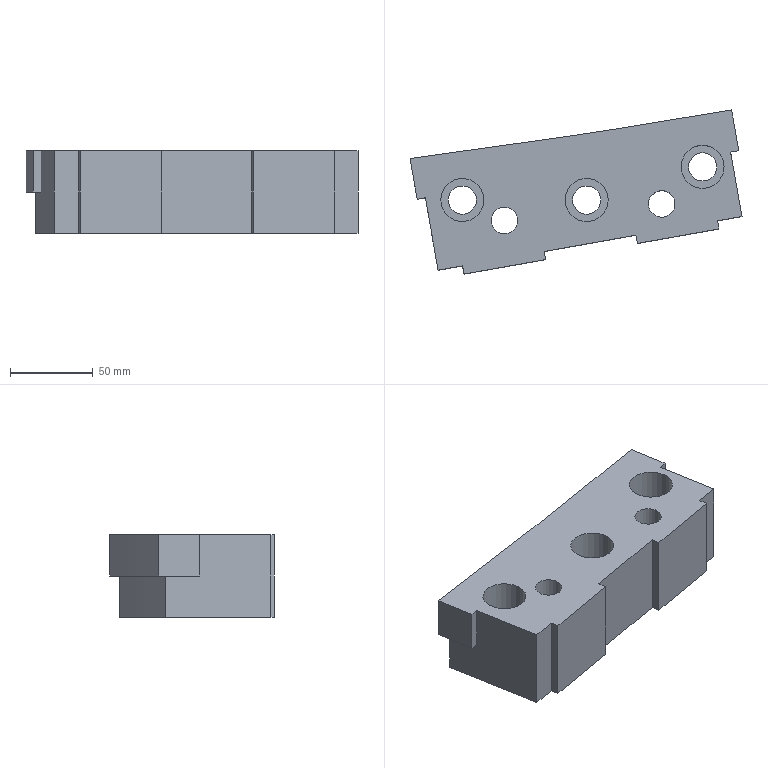Part | NX | features solid 2 | 1 solid | 31 faces | box 200.425 x 99.072 x 50 mm | volume 548993 mm3 | plane 21 | cylinder 8 | spline 2 | commonest cylinder face diameters 17 x3 26 x3 16 x2
STEP:
#1=CARTESIAN_POINT('',(8.477,507.421,0.));
#2=VERTEX_POINT('',#1);
#3=CARTESIAN_POINT('',(0.477,507.421,0.));
#4=DIRECTION('',(0.,0.,1.));
#5=DIRECTION('',(1.,0.,0.));
#6=AXIS2_PLACEMENT_3D('',#3,#4,#5);
#7=CIRCLE('',#6,8.);
#8=EDGE_CURVE('',#2,#2,#7,.T.);
#9=ORIENTED_EDGE('',*,*,#8,.F.);
#10=EDGE_LOOP('',(#9));
#11=FACE_BOUND('',#10,.T.);
#12=CARTESIAN_POINT('',(103.477,517.421,0.));
#13=VERTEX_POINT('',#12);
#14=CARTESIAN_POINT('',(95.477,517.421,0.));
#15=DIRECTION('',(0.,0.,1.));
#16=DIRECTION('',(1.,0.,0.));
#17=AXIS2_PLACEMENT_3D('',#14,#15,#16);
#18=CIRCLE('',#17,8.);
#19=EDGE_CURVE('',#13,#13,#18,.T.);
#20=ORIENTED_EDGE('',*,*,#19,.F.);
#21=EDGE_LOOP('',(#20));
#22=FACE_BOUND('',#21,.T.);
#23=CARTESIAN_POINT('',(-52.15,520.238,0.));
#24=VERTEX_POINT('',#23);
#25=CARTESIAN_POINT('',(-47.226,521.106,0.));
#26=VERTEX_POINT('',#25);
#27=CARTESIAN_POINT('',(-57.074,519.37,0.));
#28=DIRECTION('',(0.9848,0.1736,0.));
#29=VECTOR('',#28,1000.);
#30=LINE('',#27,#29);
#31=EDGE_CURVE('',#24,#26,#30,.T.);
#32=ORIENTED_EDGE('',*,*,#31,.T.);
#33=CARTESIAN_POINT('',(-39.523,477.421,0.));
#34=VERTEX_POINT('',#33);
#35=CARTESIAN_POINT('',(-39.523,477.421,0.));
#36=DIRECTION('',(-0.1736,0.9848,0.));
#37=VECTOR('',#36,1000.);
#38=LINE('',#35,#37);
#39=EDGE_CURVE('',#34,#26,#38,.T.);
#40=ORIENTED_EDGE('',*,*,#39,.F.);
#41=CARTESIAN_POINT('',(-24.751,480.026,0.));
#42=VERTEX_POINT('',#41);
#43=CARTESIAN_POINT('',(148.858,510.637,0.));
#44=DIRECTION('',(-0.9848,-0.1736,0.));
#45=VECTOR('',#44,1000.);
#46=LINE('',#43,#45);
#47=EDGE_CURVE('',#42,#34,#46,.T.);
#48=ORIENTED_EDGE('',*,*,#47,.F.);
#49=CARTESIAN_POINT('',(-23.883,475.101,0.));
#50=VERTEX_POINT('',#49);
#51=CARTESIAN_POINT('',(-24.751,480.026,0.));
#52=DIRECTION('',(0.1736,-0.9848,0.));
#53=VECTOR('',#52,1000.);
#54=LINE('',#51,#53);
#55=EDGE_CURVE('',#42,#50,#54,.T.);
#56=ORIENTED_EDGE('',*,*,#55,.T.);
#57=CARTESIAN_POINT('',(25.358,483.784,0.));
#58=VERTEX_POINT('',#57);
#59=CARTESIAN_POINT('',(25.358,483.784,0.));
#60=DIRECTION('',(-0.9848,-0.1736,0.));
#61=VECTOR('',#60,1000.);
#62=LINE('',#59,#61);
#63=EDGE_CURVE('',#58,#50,#62,.T.);
#64=ORIENTED_EDGE('',*,*,#63,.F.);
#65=CARTESIAN_POINT('',(24.49,488.708,0.));
#66=VERTEX_POINT('',#65);
#67=CARTESIAN_POINT('',(24.49,488.708,0.));
#68=DIRECTION('',(0.1736,-0.9848,0.));
#69=VECTOR('',#68,1000.);
#70=LINE('',#67,#69);
#71=EDGE_CURVE('',#66,#58,#70,.T.);
#72=ORIENTED_EDGE('',*,*,#71,.F.);
#73=CARTESIAN_POINT('',(79.921,498.482,0.));
#74=VERTEX_POINT('',#73);
#75=CARTESIAN_POINT('',(148.858,510.637,0.));
#76=DIRECTION('',(-0.9848,-0.1736,0.));
#77=VECTOR('',#76,1000.);
#78=LINE('',#75,#77);
#79=EDGE_CURVE('',#74,#66,#78,.T.);
#80=ORIENTED_EDGE('',*,*,#79,.F.);
#81=CARTESIAN_POINT('',(80.79,493.558,0.));
#82=VERTEX_POINT('',#81);
#83=CARTESIAN_POINT('',(79.921,498.482,0.));
#84=DIRECTION('',(0.1736,-0.9848,0.));
#85=VECTOR('',#84,1000.);
#86=LINE('',#83,#85);
#87=EDGE_CURVE('',#74,#82,#86,.T.);
#88=ORIENTED_EDGE('',*,*,#87,.T.);
#89=CARTESIAN_POINT('',(130.03,502.24,0.));
#90=VERTEX_POINT('',#89);
#91=CARTESIAN_POINT('',(144.802,504.845,0.));
#92=DIRECTION('',(-0.9848,-0.1736,0.));
#93=VECTOR('',#92,1000.);
#94=LINE('',#91,#93);
#95=EDGE_CURVE('',#90,#82,#94,.T.);
#96=ORIENTED_EDGE('',*,*,#95,.F.);
#97=CARTESIAN_POINT('',(129.162,507.164,0.));
#98=VERTEX_POINT('',#97);
#99=CARTESIAN_POINT('',(129.162,507.164,0.));
#100=DIRECTION('',(0.1736,-0.9848,0.));
#101=VECTOR('',#100,1000.);
#102=LINE('',#99,#101);
#103=EDGE_CURVE('',#98,#90,#102,.T.);
#104=ORIENTED_EDGE('',*,*,#103,.F.);
#105=CARTESIAN_POINT('',(143.934,509.769,0.));
#106=VERTEX_POINT('',#105);
#107=CARTESIAN_POINT('',(148.858,510.637,0.));
#108=DIRECTION('',(-0.9848,-0.1736,0.));
#109=VECTOR('',#108,1000.);
#110=LINE('',#107,#109);
#111=EDGE_CURVE('',#106,#98,#110,.T.);
#112=ORIENTED_EDGE('',*,*,#111,.F.);
#113=CARTESIAN_POINT('',(137.072,548.685,0.));
#114=VERTEX_POINT('',#113);
#115=CARTESIAN_POINT('',(143.934,509.769,0.));
#116=DIRECTION('',(-0.1736,0.9848,0.));
#117=VECTOR('',#116,1000.);
#118=LINE('',#115,#117);
#119=EDGE_CURVE('',#106,#114,#118,.T.);
#120=ORIENTED_EDGE('',*,*,#119,.T.);
#121=CARTESIAN_POINT('',(141.996,549.553,0.));
#122=VERTEX_POINT('',#121);
#123=CARTESIAN_POINT('',(146.92,550.422,0.));
#124=DIRECTION('',(-0.9848,-0.1736,0.));
#125=VECTOR('',#124,1000.);
#126=LINE('',#123,#125);
#127=EDGE_CURVE('',#122,#114,#126,.T.);
#128=ORIENTED_EDGE('',*,*,#127,.F.);
#129=CARTESIAN_POINT('',(137.655,574.174,0.));
#130=VERTEX_POINT('',#129);
#131=CARTESIAN_POINT('',(148.858,510.637,0.));
#132=DIRECTION('',(-0.1736,0.9848,0.));
#133=VECTOR('',#132,1000.);
#134=LINE('',#131,#133);
#135=EDGE_CURVE('',#122,#130,#134,.T.);
#136=ORIENTED_EDGE('',*,*,#135,.T.);
#137=CARTESIAN_POINT('',(-56.491,544.858,0.));
#138=VERTEX_POINT('',#137);
#139=CARTESIAN_POINT('',(137.655,574.174,0.));
#140=CARTESIAN_POINT('',(129.756,572.971,0.));
#141=CARTESIAN_POINT('',(112.276,570.118,0.));
#142=CARTESIAN_POINT('',(85.244,565.431,0.));
#143=CARTESIAN_POINT('',(56.452,560.795,0.));
#144=CARTESIAN_POINT('',(27.599,556.541,0.));
#145=CARTESIAN_POINT('',(-1.295,552.585,0.));
#146=CARTESIAN_POINT('',(-29.34,548.798,0.));
#147=CARTESIAN_POINT('',(-47.728,546.145,0.));
#148=CARTESIAN_POINT('',(-56.491,544.858,0.));
#149=B_SPLINE_CURVE_WITH_KNOTS('',3,(#139,#140,#141,#142,#143,#144,#145,#146,#147,#148),.UNSPECIFIED.,.F.,.F.,(4,1,1,1,1,1,1,4),(0.,0.1221,0.2706,0.4191,0.5676,0.7162,0.8647,1.),.UNSPECIFIED.);
#150=EDGE_CURVE('',#130,#138,#149,.T.);
#151=ORIENTED_EDGE('',*,*,#150,.T.);
#152=CARTESIAN_POINT('',(-44.447,476.553,0.));
#153=DIRECTION('',(-0.1736,0.9848,0.));
#154=VECTOR('',#153,1000.);
#155=LINE('',#152,#154);
#156=EDGE_CURVE('',#24,#138,#155,.T.);
#157=ORIENTED_EDGE('',*,*,#156,.F.);
#158=EDGE_LOOP('',(#32,#40,#48,#56,#64,#72,#80,#88,#96,#104,#112,#120,#128,#136,#151,#157));
#159=FACE_BOUND('',#158,.T.);
#160=CARTESIAN_POINT('',(63.122,519.794,0.));
#161=VERTEX_POINT('',#160);
#162=CARTESIAN_POINT('',(50.122,519.794,0.));
#163=DIRECTION('',(0.,0.,1.));
#164=DIRECTION('',(1.,0.,0.));
#165=AXIS2_PLACEMENT_3D('',#162,#163,#164);
#166=CIRCLE('',#165,13.);
#167=EDGE_CURVE('',#161,#161,#166,.T.);
#168=ORIENTED_EDGE('',*,*,#167,.F.);
#169=EDGE_LOOP('',(#168));
#170=FACE_BOUND('',#169,.T.);
#171=CARTESIAN_POINT('',(133.122,539.794,0.));
#172=VERTEX_POINT('',#171);
#173=CARTESIAN_POINT('',(120.122,539.794,0.));
#174=DIRECTION('',(0.,0.,1.));
#175=DIRECTION('',(1.,0.,0.));
#176=AXIS2_PLACEMENT_3D('',#173,#174,#175);
#177=CIRCLE('',#176,13.);
#178=EDGE_CURVE('',#172,#172,#177,.T.);
#179=ORIENTED_EDGE('',*,*,#178,.F.);
#180=EDGE_LOOP('',(#179));
#181=FACE_BOUND('',#180,.T.);
#182=CARTESIAN_POINT('',(-37.878,519.794,0.));
#183=VERTEX_POINT('',#182);
#184=CARTESIAN_POINT('',(-24.878,519.794,0.));
#185=DIRECTION('',(0.,0.,-1.));
#186=DIRECTION('',(-1.,0.,0.));
#187=AXIS2_PLACEMENT_3D('',#184,#185,#186);
#188=CIRCLE('',#187,13.);
#189=EDGE_CURVE('',#183,#183,#188,.T.);
#190=ORIENTED_EDGE('',*,*,#189,.T.);
#191=EDGE_LOOP('',(#190));
#192=FACE_BOUND('',#191,.T.);
#193=CARTESIAN_POINT('',(-40.143,-832.432,0.));
#194=DIRECTION('',(0.,0.,1.));
#195=DIRECTION('',(0.9962,-0.08716,0.));
#196=AXIS2_PLACEMENT_3D('',#193,#194,#195);
#197=PLANE('',#196);
#198=ADVANCED_FACE('',(#11,#22,#159,#170,#181,#192),#197,.T.);
#199=CARTESIAN_POINT('',(-52.15,520.238,-25.));
#200=VERTEX_POINT('',#199);
#201=CARTESIAN_POINT('',(-47.226,521.106,-25.));
#202=VERTEX_POINT('',#201);
#203=CARTESIAN_POINT('',(-57.074,519.37,-25.));
#204=DIRECTION('',(0.9848,0.1736,0.));
#205=VECTOR('',#204,1000.);
#206=LINE('',#203,#205);
#207=EDGE_CURVE('',#200,#202,#206,.T.);
#208=ORIENTED_EDGE('',*,*,#207,.F.);
#209=CARTESIAN_POINT('',(-56.491,544.858,-25.));
#210=VERTEX_POINT('',#209);
#211=CARTESIAN_POINT('',(-44.447,476.553,-25.));
#212=DIRECTION('',(0.1736,-0.9848,0.));
#213=VECTOR('',#212,1000.);
#214=LINE('',#211,#213);
#215=EDGE_CURVE('',#210,#200,#214,.T.);
#216=ORIENTED_EDGE('',*,*,#215,.F.);
#217=CARTESIAN_POINT('',(137.655,574.174,-25.));
#218=VERTEX_POINT('',#217);
#219=CARTESIAN_POINT('',(137.655,574.174,-25.));
#220=CARTESIAN_POINT('',(129.756,572.971,-25.));
#221=CARTESIAN_POINT('',(112.276,570.118,-25.));
#222=CARTESIAN_POINT('',(85.244,565.431,-25.));
#223=CARTESIAN_POINT('',(56.452,560.795,-25.));
#224=CARTESIAN_POINT('',(27.599,556.541,-25.));
#225=CARTESIAN_POINT('',(-1.295,552.585,-25.));
#226=CARTESIAN_POINT('',(-29.34,548.798,-25.));
#227=CARTESIAN_POINT('',(-47.728,546.145,-25.));
#228=CARTESIAN_POINT('',(-56.491,544.858,-25.));
#229=B_SPLINE_CURVE_WITH_KNOTS('',3,(#219,#220,#221,#222,#223,#224,#225,#226,#227,#228),.UNSPECIFIED.,.F.,.F.,(4,1,1,1,1,1,1,4),(0.,0.1221,0.2706,0.4191,0.5676,0.7162,0.8647,1.),.UNSPECIFIED.);
#230=EDGE_CURVE('',#210,#218,#229,.F.);
#231=ORIENTED_EDGE('',*,*,#230,.T.);
#232=CARTESIAN_POINT('',(141.996,549.553,-25.));
#233=VERTEX_POINT('',#232);
#234=CARTESIAN_POINT('',(148.858,510.637,-25.));
#235=DIRECTION('',(0.1736,-0.9848,0.));
#236=VECTOR('',#235,1000.);
#237=LINE('',#234,#236);
#238=EDGE_CURVE('',#218,#233,#237,.T.);
#239=ORIENTED_EDGE('',*,*,#238,.T.);
#240=CARTESIAN_POINT('',(137.072,548.685,-25.));
#241=VERTEX_POINT('',#240);
#242=CARTESIAN_POINT('',(146.92,550.422,-25.));
#243=DIRECTION('',(-0.9848,-0.1736,0.));
#244=VECTOR('',#243,1000.);
#245=LINE('',#242,#244);
#246=EDGE_CURVE('',#233,#241,#245,.T.);
#247=ORIENTED_EDGE('',*,*,#246,.T.);
#248=CARTESIAN_POINT('',(133.581,568.485,-25.));
#249=VERTEX_POINT('',#248);
#250=CARTESIAN_POINT('',(143.934,509.769,-25.));
#251=DIRECTION('',(0.1736,-0.9848,0.));
#252=VECTOR('',#251,1000.);
#253=LINE('',#250,#252);
#254=EDGE_CURVE('',#241,#249,#253,.F.);
#255=ORIENTED_EDGE('',*,*,#254,.T.);
#256=CARTESIAN_POINT('',(-50.673,540.656,-25.));
#257=VERTEX_POINT('',#256);
#258=CARTESIAN_POINT('',(133.581,568.485,-25.));
#259=CARTESIAN_POINT('',(118.304,566.095,-25.));
#260=CARTESIAN_POINT('',(87.745,560.699,-25.));
#261=CARTESIAN_POINT('',(41.601,553.395,-25.));
#262=CARTESIAN_POINT('',(-4.622,547.104,-25.));
#263=CARTESIAN_POINT('',(-35.327,542.893,-25.));
#264=CARTESIAN_POINT('',(-50.673,540.656,-25.));
#265=B_SPLINE_CURVE_WITH_KNOTS('',3,(#258,#259,#260,#261,#262,#263,#264),.UNSPECIFIED.,.F.,.F.,(4,1,1,1,4),(0.02498,0.2622,0.4994,0.7366,0.9738),.UNSPECIFIED.);
#266=EDGE_CURVE('',#249,#257,#265,.T.);
#267=ORIENTED_EDGE('',*,*,#266,.T.);
#268=CARTESIAN_POINT('',(-39.523,477.421,-25.));
#269=DIRECTION('',(0.1736,-0.9848,0.));
#270=VECTOR('',#269,1000.);
#271=LINE('',#268,#270);
#272=EDGE_CURVE('',#202,#257,#271,.F.);
#273=ORIENTED_EDGE('',*,*,#272,.F.);
#274=EDGE_LOOP('',(#208,#216,#231,#239,#247,#255,#267,#273));
#275=FACE_BOUND('',#274,.T.);
#276=CARTESIAN_POINT('',(-56.491,544.858,-25.));
#277=DIRECTION('',(0.,0.,-1.));
#278=DIRECTION('',(-0.9962,0.08716,0.));
#279=AXIS2_PLACEMENT_3D('',#276,#277,#278);
#280=PLANE('',#279);
#281=ADVANCED_FACE('',(#275),#280,.T.);
#282=ORIENTED_EDGE('',*,*,#135,.F.);
#283=CARTESIAN_POINT('',(141.996,549.553,-50.));
#284=DIRECTION('',(0.,0.,-1.));
#285=VECTOR('',#284,1000.);
#286=LINE('',#283,#285);
#287=EDGE_CURVE('',#122,#233,#286,.T.);
#288=ORIENTED_EDGE('',*,*,#287,.T.);
#289=ORIENTED_EDGE('',*,*,#238,.F.);
#290=CARTESIAN_POINT('',(137.655,574.174,-50.));
#291=DIRECTION('',(0.,0.,1.));
#292=VECTOR('',#291,1000.);
#293=LINE('',#290,#292);
#294=EDGE_CURVE('',#218,#130,#293,.T.);
#295=ORIENTED_EDGE('',*,*,#294,.T.);
#296=EDGE_LOOP('',(#282,#288,#289,#295));
#297=FACE_BOUND('',#296,.T.);
#298=CARTESIAN_POINT('',(148.858,510.637,-50.));
#299=DIRECTION('',(0.9848,0.1736,0.));
#300=DIRECTION('',(-0.1736,0.9848,0.));
#301=AXIS2_PLACEMENT_3D('',#298,#299,#300);
#302=PLANE('',#301);
#303=ADVANCED_FACE('',(#297),#302,.T.);
#304=CARTESIAN_POINT('',(143.934,509.769,-50.));
#305=VERTEX_POINT('',#304);
#306=CARTESIAN_POINT('',(143.934,509.769,-50.));
#307=DIRECTION('',(0.,0.,1.));
#308=VECTOR('',#307,1000.);
#309=LINE('',#306,#308);
#310=EDGE_CURVE('',#305,#106,#309,.T.);
#311=ORIENTED_EDGE('',*,*,#310,.T.);
#312=ORIENTED_EDGE('',*,*,#111,.T.);
#313=CARTESIAN_POINT('',(129.162,507.164,-50.));
#314=VERTEX_POINT('',#313);
#315=CARTESIAN_POINT('',(129.162,507.164,-50.));
#316=DIRECTION('',(0.,0.,1.));
#317=VECTOR('',#316,1000.);
#318=LINE('',#315,#317);
#319=EDGE_CURVE('',#314,#98,#318,.T.);
#320=ORIENTED_EDGE('',*,*,#319,.F.);
#321=CARTESIAN_POINT('',(148.858,510.637,-50.));
#322=DIRECTION('',(-0.9848,-0.1736,0.));
#323=VECTOR('',#322,1000.);
#324=LINE('',#321,#323);
#325=EDGE_CURVE('',#305,#314,#324,.T.);
#326=ORIENTED_EDGE('',*,*,#325,.F.);
#327=EDGE_LOOP('',(#311,#312,#320,#326));
#328=FACE_BOUND('',#327,.T.);
#329=CARTESIAN_POINT('',(148.858,510.637,-50.));
#330=DIRECTION('',(-0.1736,0.9848,0.));
#331=DIRECTION('',(-0.9848,-0.1736,0.));
#332=AXIS2_PLACEMENT_3D('',#329,#330,#331);
#333=PLANE('',#332);
#334=ADVANCED_FACE('',(#328),#333,.F.);
#335=CARTESIAN_POINT('',(8.477,507.421,-50.));
#336=VERTEX_POINT('',#335);
#337=CARTESIAN_POINT('',(0.477,507.421,-50.));
#338=DIRECTION('',(0.,0.,1.));
#339=DIRECTION('',(1.,0.,0.));
#340=AXIS2_PLACEMENT_3D('',#337,#338,#339);
#341=CIRCLE('',#340,8.);
#342=EDGE_CURVE('',#336,#336,#341,.T.);
#343=ORIENTED_EDGE('',*,*,#342,.T.);
#344=EDGE_LOOP('',(#343));
#345=FACE_BOUND('',#344,.T.);
#346=CARTESIAN_POINT('',(103.477,517.421,-50.));
#347=VERTEX_POINT('',#346);
#348=CARTESIAN_POINT('',(95.477,517.421,-50.));
#349=DIRECTION('',(0.,0.,1.));
#350=DIRECTION('',(1.,0.,0.));
#351=AXIS2_PLACEMENT_3D('',#348,#349,#350);
#352=CIRCLE('',#351,8.);
#353=EDGE_CURVE('',#347,#347,#352,.T.);
#354=ORIENTED_EDGE('',*,*,#353,.T.);
#355=EDGE_LOOP('',(#354));
#356=FACE_BOUND('',#355,.T.);
#357=CARTESIAN_POINT('',(133.581,568.485,-50.));
#358=VERTEX_POINT('',#357);
#359=CARTESIAN_POINT('',(132.49,574.671,-50.));
#360=DIRECTION('',(-0.1736,0.9848,0.));
#361=VECTOR('',#360,1000.);
#362=LINE('',#359,#361);
#363=EDGE_CURVE('',#305,#358,#362,.T.);
#364=ORIENTED_EDGE('',*,*,#363,.F.);
#365=ORIENTED_EDGE('',*,*,#325,.T.);
#366=CARTESIAN_POINT('',(130.03,502.24,-50.));
#367=VERTEX_POINT('',#366);
#368=CARTESIAN_POINT('',(129.162,507.164,-50.));
#369=DIRECTION('',(0.1736,-0.9848,0.));
#370=VECTOR('',#369,1000.);
#371=LINE('',#368,#370);
#372=EDGE_CURVE('',#314,#367,#371,.T.);
#373=ORIENTED_EDGE('',*,*,#372,.T.);
#374=CARTESIAN_POINT('',(80.79,493.558,-50.));
#375=VERTEX_POINT('',#374);
#376=CARTESIAN_POINT('',(144.802,504.845,-50.));
#377=DIRECTION('',(-0.9848,-0.1736,0.));
#378=VECTOR('',#377,1000.);
#379=LINE('',#376,#378);
#380=EDGE_CURVE('',#367,#375,#379,.T.);
#381=ORIENTED_EDGE('',*,*,#380,.T.);
#382=CARTESIAN_POINT('',(79.921,498.482,-50.));
#383=VERTEX_POINT('',#382);
#384=CARTESIAN_POINT('',(79.921,498.482,-50.));
#385=DIRECTION('',(0.1736,-0.9848,0.));
#386=VECTOR('',#385,1000.);
#387=LINE('',#384,#386);
#388=EDGE_CURVE('',#383,#375,#387,.T.);
#389=ORIENTED_EDGE('',*,*,#388,.F.);
#390=CARTESIAN_POINT('',(24.49,488.708,-50.));
#391=VERTEX_POINT('',#390);
#392=CARTESIAN_POINT('',(148.858,510.637,-50.));
#393=DIRECTION('',(-0.9848,-0.1736,0.));
#394=VECTOR('',#393,1000.);
#395=LINE('',#392,#394);
#396=EDGE_CURVE('',#383,#391,#395,.T.);
#397=ORIENTED_EDGE('',*,*,#396,.T.);
#398=CARTESIAN_POINT('',(25.358,483.784,-50.));
#399=VERTEX_POINT('',#398);
#400=CARTESIAN_POINT('',(24.49,488.708,-50.));
#401=DIRECTION('',(0.1736,-0.9848,0.));
#402=VECTOR('',#401,1000.);
#403=LINE('',#400,#402);
#404=EDGE_CURVE('',#391,#399,#403,.T.);
#405=ORIENTED_EDGE('',*,*,#404,.T.);
#406=CARTESIAN_POINT('',(-23.883,475.101,-50.));
#407=VERTEX_POINT('',#406);
#408=CARTESIAN_POINT('',(25.358,483.784,-50.));
#409=DIRECTION('',(-0.9848,-0.1736,0.));
#410=VECTOR('',#409,1000.);
#411=LINE('',#408,#410);
#412=EDGE_CURVE('',#399,#407,#411,.T.);
#413=ORIENTED_EDGE('',*,*,#412,.T.);
#414=CARTESIAN_POINT('',(-24.751,480.026,-50.));
#415=VERTEX_POINT('',#414);
#416=CARTESIAN_POINT('',(-24.751,480.026,-50.));
#417=DIRECTION('',(0.1736,-0.9848,0.));
#418=VECTOR('',#417,1000.);
#419=LINE('',#416,#418);
#420=EDGE_CURVE('',#415,#407,#419,.T.);
#421=ORIENTED_EDGE('',*,*,#420,.F.);
#422=CARTESIAN_POINT('',(-39.523,477.421,-50.));
#423=VERTEX_POINT('',#422);
#424=CARTESIAN_POINT('',(148.858,510.637,-50.));
#425=DIRECTION('',(-0.9848,-0.1736,0.));
#426=VECTOR('',#425,1000.);
#427=LINE('',#424,#426);
#428=EDGE_CURVE('',#415,#423,#427,.T.);
#429=ORIENTED_EDGE('',*,*,#428,.T.);
#430=CARTESIAN_POINT('',(-50.673,540.656,-50.));
#431=VERTEX_POINT('',#430);
#432=CARTESIAN_POINT('',(-50.967,542.323,-50.));
#433=DIRECTION('',(-0.1736,0.9848,0.));
#434=VECTOR('',#433,1000.);
#435=LINE('',#432,#434);
#436=EDGE_CURVE('',#423,#431,#435,.T.);
#437=ORIENTED_EDGE('',*,*,#436,.T.);
#438=CARTESIAN_POINT('',(-50.673,540.656,-50.));
#439=CARTESIAN_POINT('',(-48.626,540.955,-50.));
#440=CARTESIAN_POINT('',(-44.596,541.539,-50.));
#441=CARTESIAN_POINT('',(-39.713,542.24,-50.));
#442=CARTESIAN_POINT('',(-35.901,542.783,-50.));
#443=CARTESIAN_POINT('',(-33.086,543.181,-50.));
#444=CARTESIAN_POINT('',(-30.79,543.504,-50.));
#445=CARTESIAN_POINT('',(-29.182,543.729,-50.));
#446=CARTESIAN_POINT('',(-28.302,543.852,-50.));
#447=CARTESIAN_POINT('',(-27.552,543.956,-50.));
#448=CARTESIAN_POINT('',(-27.161,544.011,-50.));
#449=CARTESIAN_POINT('',(-26.486,544.104,-50.));
#450=CARTESIAN_POINT('',(-25.31,544.267,-50.));
#451=CARTESIAN_POINT('',(-23.436,544.526,-50.));
#452=CARTESIAN_POINT('',(-20.942,544.869,-50.));
#453=CARTESIAN_POINT('',(-17.266,545.373,-50.));
#454=CARTESIAN_POINT('',(-13.079,545.945,-50.));
#455=CARTESIAN_POINT('',(-8.95,546.508,-50.));
#456=CARTESIAN_POINT('',(-6.48,546.844,-50.));
#457=CARTESIAN_POINT('',(-3.855,547.2,-50.));
#458=CARTESIAN_POINT('',(-0.8949,547.603,-50.));
#459=CARTESIAN_POINT('',(3.851,548.25,-50.));
#460=CARTESIAN_POINT('',(11.737,549.332,-50.));
#461=CARTESIAN_POINT('',(19.972,550.475,-50.));
#462=CARTESIAN_POINT('',(27.393,551.518,-50.));
#463=CARTESIAN_POINT('',(31.695,552.13,-50.));
#464=CARTESIAN_POINT('',(34.937,552.595,-50.));
#465=CARTESIAN_POINT('',(37.264,552.932,-50.));
#466=CARTESIAN_POINT('',(39.13,553.203,-50.));
#467=CARTESIAN_POINT('',(40.371,553.385,-50.));
#468=CARTESIAN_POINT('',(41.1,553.492,-50.));
#469=CARTESIAN_POINT('',(41.55,553.558,-50.));
#470=CARTESIAN_POINT('',(42.339,553.675,-50.));
#471=CARTESIAN_POINT('',(43.272,553.812,-50.));
#472=CARTESIAN_POINT('',(44.961,554.063,-50.));
#473=CARTESIAN_POINT('',(47.345,554.419,-50.));
#474=CARTESIAN_POINT('',(50.219,554.851,-50.));
#475=CARTESIAN_POINT('',(54.048,555.433,-50.));
#476=CARTESIAN_POINT('',(58.838,556.169,-50.));
#477=CARTESIAN_POINT('',(66.506,557.368,-50.));
#478=CARTESIAN_POINT('',(76.095,558.903,-50.));
#479=CARTESIAN_POINT('',(87.637,560.814,-50.));
#480=CARTESIAN_POINT('',(97.202,562.433,-50.));
#481=CARTESIAN_POINT('',(104.843,563.732,-50.));
#482=CARTESIAN_POINT('',(110.63,564.726,-50.));
#483=CARTESIAN_POINT('',(116.194,565.673,-50.));
#484=CARTESIAN_POINT('',(123.825,566.938,-50.));
#485=CARTESIAN_POINT('',(129.643,567.869,-50.));
#486=CARTESIAN_POINT('',(133.581,568.485,-50.));
#487=B_SPLINE_CURVE_WITH_KNOTS('',3,(#438,#439,#440,#441,#442,#443,#444,#445,#446,#447,#448,#449,#450,#451,#452,#453,#454,#455,#456,#457,#458,#459,#460,#461,#462,#463,#464,#465,#466,#467,#468,#469,#470,#471,#472,#473,#474,#475,#476,#477,#478,#479,#480,#481,#482,#483,#484,#485,#486),.UNSPECIFIED.,.F.,.F.,(4,1,1,1,1,1,1,1,1,1,1,1,1,1,1,1,1,1,1,1,1,1,1,1,1,1,1,1,1,1,1,1,1,1,1,1,1,1,1,1,1,1,1,1,1,1,4),(0.,0.03125,0.0625,0.07812,0.09375,0.1094,0.1172,0.1211,0.125,0.1289,0.1328,0.1406,0.1562,0.1719,0.1875,0.2188,0.2344,0.2422,0.25,0.2656,0.2812,0.3125,0.375,0.4062,0.4375,0.4531,0.4688,0.4844,0.4922,0.4961,0.5,0.5039,0.5078,0.5156,0.5312,0.5469,0.5625,0.5938,0.625,0.6875,0.75,0.8125,0.8438,0.875,0.9062,0.9375,1.),.UNSPECIFIED.);
#488=EDGE_CURVE('',#358,#431,#487,.F.);
#489=ORIENTED_EDGE('',*,*,#488,.F.);
#490=EDGE_LOOP('',(#364,#365,#373,#381,#389,#397,#405,#413,#421,#429,#437,#489));
#491=FACE_BOUND('',#490,.T.);
#492=CARTESIAN_POINT('',(41.622,519.794,-50.));
#493=VERTEX_POINT('',#492);
#494=CARTESIAN_POINT('',(50.122,519.794,-50.));
#495=DIRECTION('',(0.,0.,-1.));
#496=DIRECTION('',(-1.,0.,0.));
#497=AXIS2_PLACEMENT_3D('',#494,#495,#496);
#498=CIRCLE('',#497,8.5);
#499=EDGE_CURVE('',#493,#493,#498,.T.);
#500=ORIENTED_EDGE('',*,*,#499,.F.);
#501=EDGE_LOOP('',(#500));
#502=FACE_BOUND('',#501,.T.);
#503=CARTESIAN_POINT('',(111.622,539.794,-50.));
#504=VERTEX_POINT('',#503);
#505=CARTESIAN_POINT('',(120.122,539.794,-50.));
#506=DIRECTION('',(0.,0.,-1.));
#507=DIRECTION('',(-1.,0.,0.));
#508=AXIS2_PLACEMENT_3D('',#505,#506,#507);
#509=CIRCLE('',#508,8.5);
#510=EDGE_CURVE('',#504,#504,#509,.T.);
#511=ORIENTED_EDGE('',*,*,#510,.F.);
#512=EDGE_LOOP('',(#511));
#513=FACE_BOUND('',#512,.T.);
#514=CARTESIAN_POINT('',(-33.378,519.794,-50.));
#515=VERTEX_POINT('',#514);
#516=CARTESIAN_POINT('',(-24.878,519.794,-50.));
#517=DIRECTION('',(0.,0.,-1.));
#518=DIRECTION('',(-1.,0.,0.));
#519=AXIS2_PLACEMENT_3D('',#516,#517,#518);
#520=CIRCLE('',#519,8.5);
#521=EDGE_CURVE('',#515,#515,#520,.T.);
#522=ORIENTED_EDGE('',*,*,#521,.F.);
#523=EDGE_LOOP('',(#522));
#524=FACE_BOUND('',#523,.T.);
#525=CARTESIAN_POINT('',(-40.143,-832.432,-50.));
#526=DIRECTION('',(0.,0.,1.));
#527=DIRECTION('',(0.9962,-0.08716,0.));
#528=AXIS2_PLACEMENT_3D('',#525,#526,#527);
#529=PLANE('',#528);
#530=ADVANCED_FACE('',(#345,#356,#491,#502,#513,#524),#529,.F.);
#531=CARTESIAN_POINT('',(-11.878,519.794,-25.));
#532=VERTEX_POINT('',#531);
#533=CARTESIAN_POINT('',(-24.878,519.794,-25.));
#534=DIRECTION('',(0.,0.,1.));
#535=DIRECTION('',(1.,0.,0.));
#536=AXIS2_PLACEMENT_3D('',#533,#534,#535);
#537=CIRCLE('',#536,13.);
#538=EDGE_CURVE('',#532,#532,#537,.T.);
#539=ORIENTED_EDGE('',*,*,#538,.T.);
#540=EDGE_LOOP('',(#539));
#541=FACE_BOUND('',#540,.T.);
#542=CARTESIAN_POINT('',(-33.378,519.794,-25.));
#543=VERTEX_POINT('',#542);
#544=CARTESIAN_POINT('',(-24.878,519.794,-25.));
#545=DIRECTION('',(0.,0.,-1.));
#546=DIRECTION('',(-1.,0.,0.));
#547=AXIS2_PLACEMENT_3D('',#544,#545,#546);
#548=CIRCLE('',#547,8.5);
#549=EDGE_CURVE('',#543,#543,#548,.F.);
#550=ORIENTED_EDGE('',*,*,#549,.F.);
#551=EDGE_LOOP('',(#550));
#552=FACE_BOUND('',#551,.T.);
#553=CARTESIAN_POINT('',(-24.878,519.794,-25.));
#554=DIRECTION('',(0.,0.,-1.));
#555=DIRECTION('',(-1.,0.,0.));
#556=AXIS2_PLACEMENT_3D('',#553,#554,#555);
#557=PLANE('',#556);
#558=ADVANCED_FACE('',(#541,#552),#557,.F.);
#559=ORIENTED_EDGE('',*,*,#521,.T.);
#560=EDGE_LOOP('',(#559));
#561=FACE_BOUND('',#560,.T.);
#562=ORIENTED_EDGE('',*,*,#549,.T.);
#563=EDGE_LOOP('',(#562));
#564=FACE_BOUND('',#563,.T.);
#565=CARTESIAN_POINT('',(-24.878,519.794,-75.));
#566=DIRECTION('',(0.,0.,1.));
#567=DIRECTION('',(1.,0.,0.));
#568=AXIS2_PLACEMENT_3D('',#565,#566,#567);
#569=CYLINDRICAL_SURFACE('',#568,8.5);
#570=ADVANCED_FACE('',(#561,#564),#569,.F.);
#571=ORIENTED_EDGE('',*,*,#189,.F.);
#572=EDGE_LOOP('',(#571));
#573=FACE_BOUND('',#572,.T.);
#574=ORIENTED_EDGE('',*,*,#538,.F.);
#575=EDGE_LOOP('',(#574));
#576=FACE_BOUND('',#575,.T.);
#577=CARTESIAN_POINT('',(-24.878,519.794,-25.));
#578=DIRECTION('',(0.,0.,1.));
#579=DIRECTION('',(1.,0.,0.));
#580=AXIS2_PLACEMENT_3D('',#577,#578,#579);
#581=CYLINDRICAL_SURFACE('',#580,13.);
#582=ADVANCED_FACE('',(#573,#576),#581,.F.);
#583=ORIENTED_EDGE('',*,*,#215,.T.);
#584=CARTESIAN_POINT('',(-52.15,520.238,-50.));
#585=DIRECTION('',(0.,0.,1.));
#586=VECTOR('',#585,1000.);
#587=LINE('',#584,#586);
#588=EDGE_CURVE('',#200,#24,#587,.T.);
#589=ORIENTED_EDGE('',*,*,#588,.T.);
#590=ORIENTED_EDGE('',*,*,#156,.T.);
#591=CARTESIAN_POINT('',(-56.491,544.858,-50.));
#592=DIRECTION('',(0.,0.,1.));
#593=VECTOR('',#592,1000.);
#594=LINE('',#591,#593);
#595=EDGE_CURVE('',#210,#138,#594,.T.);
#596=ORIENTED_EDGE('',*,*,#595,.F.);
#597=EDGE_LOOP('',(#583,#589,#590,#596));
#598=FACE_BOUND('',#597,.T.);
#599=CARTESIAN_POINT('',(-44.447,476.553,-50.));
#600=DIRECTION('',(0.9848,0.1736,0.));
#601=DIRECTION('',(-0.1736,0.9848,0.));
#602=AXIS2_PLACEMENT_3D('',#599,#600,#601);
#603=PLANE('',#602);
#604=ADVANCED_FACE('',(#598),#603,.F.);
#605=ORIENTED_EDGE('',*,*,#230,.F.);
#606=ORIENTED_EDGE('',*,*,#595,.T.);
#607=ORIENTED_EDGE('',*,*,#150,.F.);
#608=ORIENTED_EDGE('',*,*,#294,.F.);
#609=EDGE_LOOP('',(#605,#606,#607,#608));
#610=FACE_BOUND('',#609,.T.);
#611=CARTESIAN_POINT('',(137.655,574.174,-25.));
#612=CARTESIAN_POINT('',(137.655,574.174,0.));
#613=CARTESIAN_POINT('',(121.479,571.711,-25.));
#614=CARTESIAN_POINT('',(121.479,571.711,0.));
#615=CARTESIAN_POINT('',(89.246,566.024,-25.));
#616=CARTESIAN_POINT('',(89.246,566.024,0.));
#617=CARTESIAN_POINT('',(40.765,558.301,-25.));
#618=CARTESIAN_POINT('',(40.765,558.301,0.));
#619=CARTESIAN_POINT('',(-7.885,551.726,-25.));
#620=CARTESIAN_POINT('',(-7.885,551.726,0.));
#621=CARTESIAN_POINT('',(-40.302,547.236,-25.));
#622=CARTESIAN_POINT('',(-40.302,547.236,0.));
#623=CARTESIAN_POINT('',(-56.491,544.858,-25.));
#624=CARTESIAN_POINT('',(-56.491,544.858,0.));
#625=B_SPLINE_SURFACE_WITH_KNOTS('',3,1,((#611,#612),(#613,#614),(#615,#616),(#617,#618),(#619,#620),(#621,#622),(#623,#624)),.SURF_OF_LINEAR_EXTRUSION.,.F.,.F.,.F.,(4,1,1,1,4),(2,2),(0.,0.25,0.5,0.75,1.),(0.,1.),.UNSPECIFIED.);
#626=ADVANCED_FACE('',(#610),#625,.T.);
#627=ORIENTED_EDGE('',*,*,#254,.F.);
#628=CARTESIAN_POINT('',(137.072,548.685,-50.));
#629=DIRECTION('',(0.,0.,1.));
#630=VECTOR('',#629,1000.);
#631=LINE('',#628,#630);
#632=EDGE_CURVE('',#241,#114,#631,.T.);
#633=ORIENTED_EDGE('',*,*,#632,.T.);
#634=ORIENTED_EDGE('',*,*,#119,.F.);
#635=ORIENTED_EDGE('',*,*,#310,.F.);
#636=ORIENTED_EDGE('',*,*,#363,.T.);
#637=CARTESIAN_POINT('',(133.581,568.485,-37.5));
#638=DIRECTION('',(0.,0.,-1.));
#639=VECTOR('',#638,1000.);
#640=LINE('',#637,#639);
#641=EDGE_CURVE('',#249,#358,#640,.T.);
#642=ORIENTED_EDGE('',*,*,#641,.F.);
#643=EDGE_LOOP('',(#627,#633,#634,#635,#636,#642));
#644=FACE_BOUND('',#643,.T.);
#645=CARTESIAN_POINT('',(143.934,509.769,-25.));
#646=DIRECTION('',(-0.9848,-0.1736,0.));
#647=DIRECTION('',(0.1736,-0.9848,0.));
#648=AXIS2_PLACEMENT_3D('',#645,#646,#647);
#649=PLANE('',#648);
#650=ADVANCED_FACE('',(#644),#649,.F.);
#651=ORIENTED_EDGE('',*,*,#436,.F.);
#652=CARTESIAN_POINT('',(-39.523,477.421,-50.));
#653=DIRECTION('',(0.,0.,1.));
#654=VECTOR('',#653,1000.);
#655=LINE('',#652,#654);
#656=EDGE_CURVE('',#423,#34,#655,.T.);
#657=ORIENTED_EDGE('',*,*,#656,.T.);
#658=ORIENTED_EDGE('',*,*,#39,.T.);
#659=CARTESIAN_POINT('',(-47.226,521.106,-50.));
#660=DIRECTION('',(0.,0.,1.));
#661=VECTOR('',#660,1000.);
#662=LINE('',#659,#661);
#663=EDGE_CURVE('',#202,#26,#662,.T.);
#664=ORIENTED_EDGE('',*,*,#663,.F.);
#665=ORIENTED_EDGE('',*,*,#272,.T.);
#666=CARTESIAN_POINT('',(-50.673,540.656,-37.5));
#667=DIRECTION('',(0.,0.,-1.));
#668=VECTOR('',#667,1000.);
#669=LINE('',#666,#668);
#670=EDGE_CURVE('',#257,#431,#669,.T.);
#671=ORIENTED_EDGE('',*,*,#670,.T.);
#672=EDGE_LOOP('',(#651,#657,#658,#664,#665,#671));
#673=FACE_BOUND('',#672,.T.);
#674=CARTESIAN_POINT('',(-39.523,477.421,-25.));
#675=DIRECTION('',(-0.9848,-0.1736,0.));
#676=DIRECTION('',(0.1736,-0.9848,0.));
#677=AXIS2_PLACEMENT_3D('',#674,#675,#676);
#678=PLANE('',#677);
#679=ADVANCED_FACE('',(#673),#678,.T.);
#680=ORIENTED_EDGE('',*,*,#266,.F.);
#681=ORIENTED_EDGE('',*,*,#641,.T.);
#682=ORIENTED_EDGE('',*,*,#488,.T.);
#683=ORIENTED_EDGE('',*,*,#670,.F.);
#684=EDGE_LOOP('',(#680,#681,#682,#683));
#685=FACE_BOUND('',#684,.T.);
#686=CARTESIAN_POINT('',(133.581,568.485,-25.));
#687=CARTESIAN_POINT('',(133.581,568.485,-50.));
#688=CARTESIAN_POINT('',(118.304,566.095,-25.));
#689=CARTESIAN_POINT('',(118.304,566.095,-50.));
#690=CARTESIAN_POINT('',(87.745,560.699,-25.));
#691=CARTESIAN_POINT('',(87.745,560.699,-50.));
#692=CARTESIAN_POINT('',(41.601,553.395,-25.));
#693=CARTESIAN_POINT('',(41.601,553.395,-50.));
#694=CARTESIAN_POINT('',(-4.622,547.104,-25.));
#695=CARTESIAN_POINT('',(-4.622,547.104,-50.));
#696=CARTESIAN_POINT('',(-35.327,542.893,-25.));
#697=CARTESIAN_POINT('',(-35.327,542.893,-50.));
#698=CARTESIAN_POINT('',(-50.673,540.656,-25.));
#699=CARTESIAN_POINT('',(-50.673,540.656,-50.));
#700=B_SPLINE_SURFACE_WITH_KNOTS('',3,1,((#686,#687),(#688,#689),(#690,#691),(#692,#693),(#694,#695),(#696,#697),(#698,#699)),.SURF_OF_LINEAR_EXTRUSION.,.F.,.F.,.F.,(4,1,1,1,4),(2,2),(0.02498,0.2622,0.4994,0.7366,0.9738),(0.,1.),.UNSPECIFIED.);
#701=ADVANCED_FACE('',(#685),#700,.F.);
#702=CARTESIAN_POINT('',(133.122,539.794,-25.));
#703=VERTEX_POINT('',#702);
#704=CARTESIAN_POINT('',(120.122,539.794,-25.));
#705=DIRECTION('',(0.,0.,1.));
#706=DIRECTION('',(1.,0.,0.));
#707=AXIS2_PLACEMENT_3D('',#704,#705,#706);
#708=CIRCLE('',#707,13.);
#709=EDGE_CURVE('',#703,#703,#708,.T.);
#710=ORIENTED_EDGE('',*,*,#709,.F.);
#711=EDGE_LOOP('',(#710));
#712=FACE_BOUND('',#711,.T.);
#713=ORIENTED_EDGE('',*,*,#178,.T.);
#714=EDGE_LOOP('',(#713));
#715=FACE_BOUND('',#714,.T.);
#716=CARTESIAN_POINT('',(120.122,539.794,-25.));
#717=DIRECTION('',(0.,0.,1.));
#718=DIRECTION('',(1.,0.,0.));
#719=AXIS2_PLACEMENT_3D('',#716,#717,#718);
#720=CYLINDRICAL_SURFACE('',#719,13.);
#721=ADVANCED_FACE('',(#712,#715),#720,.F.);
#722=CARTESIAN_POINT('',(111.622,539.794,-25.));
#723=VERTEX_POINT('',#722);
#724=CARTESIAN_POINT('',(120.122,539.794,-25.));
#725=DIRECTION('',(0.,0.,-1.));
#726=DIRECTION('',(-1.,0.,0.));
#727=AXIS2_PLACEMENT_3D('',#724,#725,#726);
#728=CIRCLE('',#727,8.5);
#729=EDGE_CURVE('',#723,#723,#728,.F.);
#730=ORIENTED_EDGE('',*,*,#729,.F.);
#731=EDGE_LOOP('',(#730));
#732=FACE_BOUND('',#731,.T.);
#733=ORIENTED_EDGE('',*,*,#709,.T.);
#734=EDGE_LOOP('',(#733));
#735=FACE_BOUND('',#734,.T.);
#736=CARTESIAN_POINT('',(120.122,539.794,-25.));
#737=DIRECTION('',(0.,0.,-1.));
#738=DIRECTION('',(-1.,0.,0.));
#739=AXIS2_PLACEMENT_3D('',#736,#737,#738);
#740=PLANE('',#739);
#741=ADVANCED_FACE('',(#732,#735),#740,.F.);
#742=ORIENTED_EDGE('',*,*,#510,.T.);
#743=EDGE_LOOP('',(#742));
#744=FACE_BOUND('',#743,.T.);
#745=ORIENTED_EDGE('',*,*,#729,.T.);
#746=EDGE_LOOP('',(#745));
#747=FACE_BOUND('',#746,.T.);
#748=CARTESIAN_POINT('',(120.122,539.794,-75.));
#749=DIRECTION('',(0.,0.,1.));
#750=DIRECTION('',(1.,0.,0.));
#751=AXIS2_PLACEMENT_3D('',#748,#749,#750);
#752=CYLINDRICAL_SURFACE('',#751,8.5);
#753=ADVANCED_FACE('',(#744,#747),#752,.F.);
#754=CARTESIAN_POINT('',(63.122,519.794,-25.));
#755=VERTEX_POINT('',#754);
#756=CARTESIAN_POINT('',(50.122,519.794,-25.));
#757=DIRECTION('',(0.,0.,1.));
#758=DIRECTION('',(1.,0.,0.));
#759=AXIS2_PLACEMENT_3D('',#756,#757,#758);
#760=CIRCLE('',#759,13.);
#761=EDGE_CURVE('',#755,#755,#760,.T.);
#762=ORIENTED_EDGE('',*,*,#761,.F.);
#763=EDGE_LOOP('',(#762));
#764=FACE_BOUND('',#763,.T.);
#765=ORIENTED_EDGE('',*,*,#167,.T.);
#766=EDGE_LOOP('',(#765));
#767=FACE_BOUND('',#766,.T.);
#768=CARTESIAN_POINT('',(50.122,519.794,-25.));
#769=DIRECTION('',(0.,0.,1.));
#770=DIRECTION('',(1.,0.,0.));
#771=AXIS2_PLACEMENT_3D('',#768,#769,#770);
#772=CYLINDRICAL_SURFACE('',#771,13.);
#773=ADVANCED_FACE('',(#764,#767),#772,.F.);
#774=ORIENTED_EDGE('',*,*,#499,.T.);
#775=EDGE_LOOP('',(#774));
#776=FACE_BOUND('',#775,.T.);
#777=CARTESIAN_POINT('',(41.622,519.794,-25.));
#778=VERTEX_POINT('',#777);
#779=CARTESIAN_POINT('',(50.122,519.794,-25.));
#780=DIRECTION('',(0.,0.,-1.));
#781=DIRECTION('',(-1.,0.,0.));
#782=AXIS2_PLACEMENT_3D('',#779,#780,#781);
#783=CIRCLE('',#782,8.5);
#784=EDGE_CURVE('',#778,#778,#783,.F.);
#785=ORIENTED_EDGE('',*,*,#784,.T.);
#786=EDGE_LOOP('',(#785));
#787=FACE_BOUND('',#786,.T.);
#788=CARTESIAN_POINT('',(50.122,519.794,-75.));
#789=DIRECTION('',(0.,0.,1.));
#790=DIRECTION('',(1.,0.,0.));
#791=AXIS2_PLACEMENT_3D('',#788,#789,#790);
#792=CYLINDRICAL_SURFACE('',#791,8.5);
#793=ADVANCED_FACE('',(#776,#787),#792,.F.);
#794=ORIENTED_EDGE('',*,*,#784,.F.);
#795=EDGE_LOOP('',(#794));
#796=FACE_BOUND('',#795,.T.);
#797=ORIENTED_EDGE('',*,*,#761,.T.);
#798=EDGE_LOOP('',(#797));
#799=FACE_BOUND('',#798,.T.);
#800=CARTESIAN_POINT('',(50.122,519.794,-25.));
#801=DIRECTION('',(0.,0.,-1.));
#802=DIRECTION('',(-1.,0.,0.));
#803=AXIS2_PLACEMENT_3D('',#800,#801,#802);
#804=PLANE('',#803);
#805=ADVANCED_FACE('',(#796,#799),#804,.F.);
#806=CARTESIAN_POINT('',(130.03,502.24,-50.));
#807=DIRECTION('',(0.,0.,1.));
#808=VECTOR('',#807,1000.);
#809=LINE('',#806,#808);
#810=EDGE_CURVE('',#367,#90,#809,.T.);
#811=ORIENTED_EDGE('',*,*,#810,.F.);
#812=ORIENTED_EDGE('',*,*,#372,.F.);
#813=ORIENTED_EDGE('',*,*,#319,.T.);
#814=ORIENTED_EDGE('',*,*,#103,.T.);
#815=EDGE_LOOP('',(#811,#812,#813,#814));
#816=FACE_BOUND('',#815,.T.);
#817=CARTESIAN_POINT('',(129.162,507.164,-50.));
#818=DIRECTION('',(0.9848,0.1736,0.));
#819=DIRECTION('',(-0.1736,0.9848,0.));
#820=AXIS2_PLACEMENT_3D('',#817,#818,#819);
#821=PLANE('',#820);
#822=ADVANCED_FACE('',(#816),#821,.T.);
#823=ORIENTED_EDGE('',*,*,#95,.T.);
#824=CARTESIAN_POINT('',(80.79,493.558,-50.));
#825=DIRECTION('',(0.,0.,1.));
#826=VECTOR('',#825,1000.);
#827=LINE('',#824,#826);
#828=EDGE_CURVE('',#375,#82,#827,.T.);
#829=ORIENTED_EDGE('',*,*,#828,.F.);
#830=ORIENTED_EDGE('',*,*,#380,.F.);
#831=ORIENTED_EDGE('',*,*,#810,.T.);
#832=EDGE_LOOP('',(#823,#829,#830,#831));
#833=FACE_BOUND('',#832,.T.);
#834=CARTESIAN_POINT('',(144.802,504.845,-50.));
#835=DIRECTION('',(-0.1736,0.9848,0.));
#836=DIRECTION('',(-0.9848,-0.1736,0.));
#837=AXIS2_PLACEMENT_3D('',#834,#835,#836);
#838=PLANE('',#837);
#839=ADVANCED_FACE('',(#833),#838,.F.);
#840=ORIENTED_EDGE('',*,*,#828,.T.);
#841=ORIENTED_EDGE('',*,*,#87,.F.);
#842=CARTESIAN_POINT('',(79.921,498.482,-50.));
#843=DIRECTION('',(0.,0.,1.));
#844=VECTOR('',#843,1000.);
#845=LINE('',#842,#844);
#846=EDGE_CURVE('',#383,#74,#845,.T.);
#847=ORIENTED_EDGE('',*,*,#846,.F.);
#848=ORIENTED_EDGE('',*,*,#388,.T.);
#849=EDGE_LOOP('',(#840,#841,#847,#848));
#850=FACE_BOUND('',#849,.T.);
#851=CARTESIAN_POINT('',(79.921,498.482,-50.));
#852=DIRECTION('',(0.9848,0.1736,0.));
#853=DIRECTION('',(-0.1736,0.9848,0.));
#854=AXIS2_PLACEMENT_3D('',#851,#852,#853);
#855=PLANE('',#854);
#856=ADVANCED_FACE('',(#850),#855,.F.);
#857=ORIENTED_EDGE('',*,*,#846,.T.);
#858=ORIENTED_EDGE('',*,*,#79,.T.);
#859=CARTESIAN_POINT('',(24.49,488.708,-50.));
#860=DIRECTION('',(0.,0.,1.));
#861=VECTOR('',#860,1000.);
#862=LINE('',#859,#861);
#863=EDGE_CURVE('',#391,#66,#862,.T.);
#864=ORIENTED_EDGE('',*,*,#863,.F.);
#865=ORIENTED_EDGE('',*,*,#396,.F.);
#866=EDGE_LOOP('',(#857,#858,#864,#865));
#867=FACE_BOUND('',#866,.T.);
#868=CARTESIAN_POINT('',(148.858,510.637,-50.));
#869=DIRECTION('',(-0.1736,0.9848,0.));
#870=DIRECTION('',(-0.9848,-0.1736,0.));
#871=AXIS2_PLACEMENT_3D('',#868,#869,#870);
#872=PLANE('',#871);
#873=ADVANCED_FACE('',(#867),#872,.F.);
#874=CARTESIAN_POINT('',(25.358,483.784,-50.));
#875=DIRECTION('',(0.,0.,1.));
#876=VECTOR('',#875,1000.);
#877=LINE('',#874,#876);
#878=EDGE_CURVE('',#399,#58,#877,.T.);
#879=ORIENTED_EDGE('',*,*,#878,.F.);
#880=ORIENTED_EDGE('',*,*,#404,.F.);
#881=ORIENTED_EDGE('',*,*,#863,.T.);
#882=ORIENTED_EDGE('',*,*,#71,.T.);
#883=EDGE_LOOP('',(#879,#880,#881,#882));
#884=FACE_BOUND('',#883,.T.);
#885=CARTESIAN_POINT('',(24.49,488.708,-50.));
#886=DIRECTION('',(0.9848,0.1736,0.));
#887=DIRECTION('',(-0.1736,0.9848,0.));
#888=AXIS2_PLACEMENT_3D('',#885,#886,#887);
#889=PLANE('',#888);
#890=ADVANCED_FACE('',(#884),#889,.T.);
#891=ORIENTED_EDGE('',*,*,#63,.T.);
#892=CARTESIAN_POINT('',(-23.883,475.101,-50.));
#893=DIRECTION('',(0.,0.,1.));
#894=VECTOR('',#893,1000.);
#895=LINE('',#892,#894);
#896=EDGE_CURVE('',#407,#50,#895,.T.);
#897=ORIENTED_EDGE('',*,*,#896,.F.);
#898=ORIENTED_EDGE('',*,*,#412,.F.);
#899=ORIENTED_EDGE('',*,*,#878,.T.);
#900=EDGE_LOOP('',(#891,#897,#898,#899));
#901=FACE_BOUND('',#900,.T.);
#902=CARTESIAN_POINT('',(25.358,483.784,-50.));
#903=DIRECTION('',(-0.1736,0.9848,0.));
#904=DIRECTION('',(-0.9848,-0.1736,0.));
#905=AXIS2_PLACEMENT_3D('',#902,#903,#904);
#906=PLANE('',#905);
#907=ADVANCED_FACE('',(#901),#906,.F.);
#908=ORIENTED_EDGE('',*,*,#896,.T.);
#909=ORIENTED_EDGE('',*,*,#55,.F.);
#910=CARTESIAN_POINT('',(-24.751,480.026,-50.));
#911=DIRECTION('',(0.,0.,1.));
#912=VECTOR('',#911,1000.);
#913=LINE('',#910,#912);
#914=EDGE_CURVE('',#415,#42,#913,.T.);
#915=ORIENTED_EDGE('',*,*,#914,.F.);
#916=ORIENTED_EDGE('',*,*,#420,.T.);
#917=EDGE_LOOP('',(#908,#909,#915,#916));
#918=FACE_BOUND('',#917,.T.);
#919=CARTESIAN_POINT('',(-24.751,480.026,-50.));
#920=DIRECTION('',(0.9848,0.1736,0.));
#921=DIRECTION('',(-0.1736,0.9848,0.));
#922=AXIS2_PLACEMENT_3D('',#919,#920,#921);
#923=PLANE('',#922);
#924=ADVANCED_FACE('',(#918),#923,.F.);
#925=ORIENTED_EDGE('',*,*,#47,.T.);
#926=ORIENTED_EDGE('',*,*,#656,.F.);
#927=ORIENTED_EDGE('',*,*,#428,.F.);
#928=ORIENTED_EDGE('',*,*,#914,.T.);
#929=EDGE_LOOP('',(#925,#926,#927,#928));
#930=FACE_BOUND('',#929,.T.);
#931=CARTESIAN_POINT('',(148.858,510.637,-50.));
#932=DIRECTION('',(-0.1736,0.9848,0.));
#933=DIRECTION('',(-0.9848,-0.1736,0.));
#934=AXIS2_PLACEMENT_3D('',#931,#932,#933);
#935=PLANE('',#934);
#936=ADVANCED_FACE('',(#930),#935,.F.);
#937=ORIENTED_EDGE('',*,*,#127,.T.);
#938=ORIENTED_EDGE('',*,*,#632,.F.);
#939=ORIENTED_EDGE('',*,*,#246,.F.);
#940=ORIENTED_EDGE('',*,*,#287,.F.);
#941=EDGE_LOOP('',(#937,#938,#939,#940));
#942=FACE_BOUND('',#941,.T.);
#943=CARTESIAN_POINT('',(146.92,550.422,-50.));
#944=DIRECTION('',(0.1736,-0.9848,0.));
#945=DIRECTION('',(0.9848,0.1736,0.));
#946=AXIS2_PLACEMENT_3D('',#943,#944,#945);
#947=PLANE('',#946);
#948=ADVANCED_FACE('',(#942),#947,.T.);
#949=ORIENTED_EDGE('',*,*,#207,.T.);
#950=ORIENTED_EDGE('',*,*,#663,.T.);
#951=ORIENTED_EDGE('',*,*,#31,.F.);
#952=ORIENTED_EDGE('',*,*,#588,.F.);
#953=EDGE_LOOP('',(#949,#950,#951,#952));
#954=FACE_BOUND('',#953,.T.);
#955=CARTESIAN_POINT('',(-57.074,519.37,-50.));
#956=DIRECTION('',(-0.1736,0.9848,0.));
#957=DIRECTION('',(-0.9848,-0.1736,0.));
#958=AXIS2_PLACEMENT_3D('',#955,#956,#957);
#959=PLANE('',#958);
#960=ADVANCED_FACE('',(#954),#959,.F.);
#961=ORIENTED_EDGE('',*,*,#19,.T.);
#962=EDGE_LOOP('',(#961));
#963=FACE_BOUND('',#962,.T.);
#964=ORIENTED_EDGE('',*,*,#353,.F.);
#965=EDGE_LOOP('',(#964));
#966=FACE_BOUND('',#965,.T.);
#967=CARTESIAN_POINT('',(95.477,517.421,50.));
#968=DIRECTION('',(0.,0.,-1.));
#969=DIRECTION('',(-1.,0.,0.));
#970=AXIS2_PLACEMENT_3D('',#967,#968,#969);
#971=CYLINDRICAL_SURFACE('',#970,8.);
#972=ADVANCED_FACE('',(#963,#966),#971,.F.);
#973=ORIENTED_EDGE('',*,*,#8,.T.);
#974=EDGE_LOOP('',(#973));
#975=FACE_BOUND('',#974,.T.);
#976=ORIENTED_EDGE('',*,*,#342,.F.);
#977=EDGE_LOOP('',(#976));
#978=FACE_BOUND('',#977,.T.);
#979=CARTESIAN_POINT('',(0.477,507.421,50.));
#980=DIRECTION('',(0.,0.,-1.));
#981=DIRECTION('',(-1.,0.,0.));
#982=AXIS2_PLACEMENT_3D('',#979,#980,#981);
#983=CYLINDRICAL_SURFACE('',#982,8.);
#984=ADVANCED_FACE('',(#975,#978),#983,.F.);
#985=CLOSED_SHELL('',(#198,#281,#303,#334,#530,#558,#570,#582,#604,#626,#650,#679,#701,#721,#741,#753,#773,#793,#805,#822,#839,#856,#873,#890,#907,#924,#936,#948,#960,#972,#984));
#986=MANIFOLD_SOLID_BREP('',#985);
#987=(LENGTH_UNIT()NAMED_UNIT(*)SI_UNIT(.MILLI.,.METRE.));
#988=UNCERTAINTY_MEASURE_WITH_UNIT(LENGTH_MEASURE(0.0508),#987,'','');
#989=(NAMED_UNIT(*)PLANE_ANGLE_UNIT()SI_UNIT($,.RADIAN.));
#990=(NAMED_UNIT(*)SI_UNIT($,.STERADIAN.)SOLID_ANGLE_UNIT());
#991=(GEOMETRIC_REPRESENTATION_CONTEXT(3)GLOBAL_UNCERTAINTY_ASSIGNED_CONTEXT((#988))GLOBAL_UNIT_ASSIGNED_CONTEXT((#987,#989,#990))REPRESENTATION_CONTEXT('',''));
#992=ADVANCED_BREP_SHAPE_REPRESENTATION('',(#986),#991);